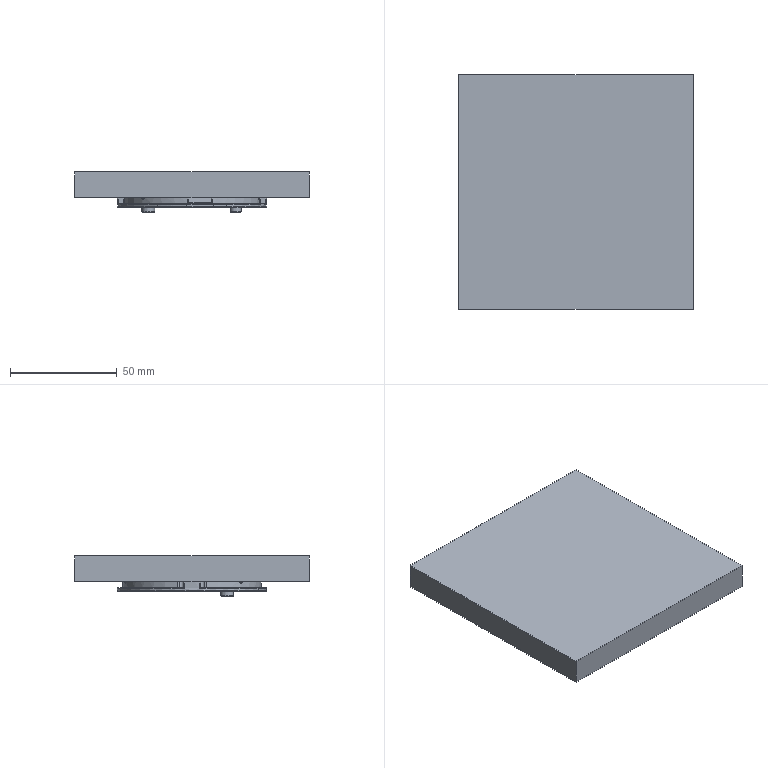Part | 3 solids | 345 faces | box 110 x 110 x 18.8 mm | volume 153469 mm3 | plane 122 | cone 119 | cylinder 104 | commonest cylinder face diameters 2 x45 1 x16 3 x10 60.8 x6 64.8 x6 2.5 x5